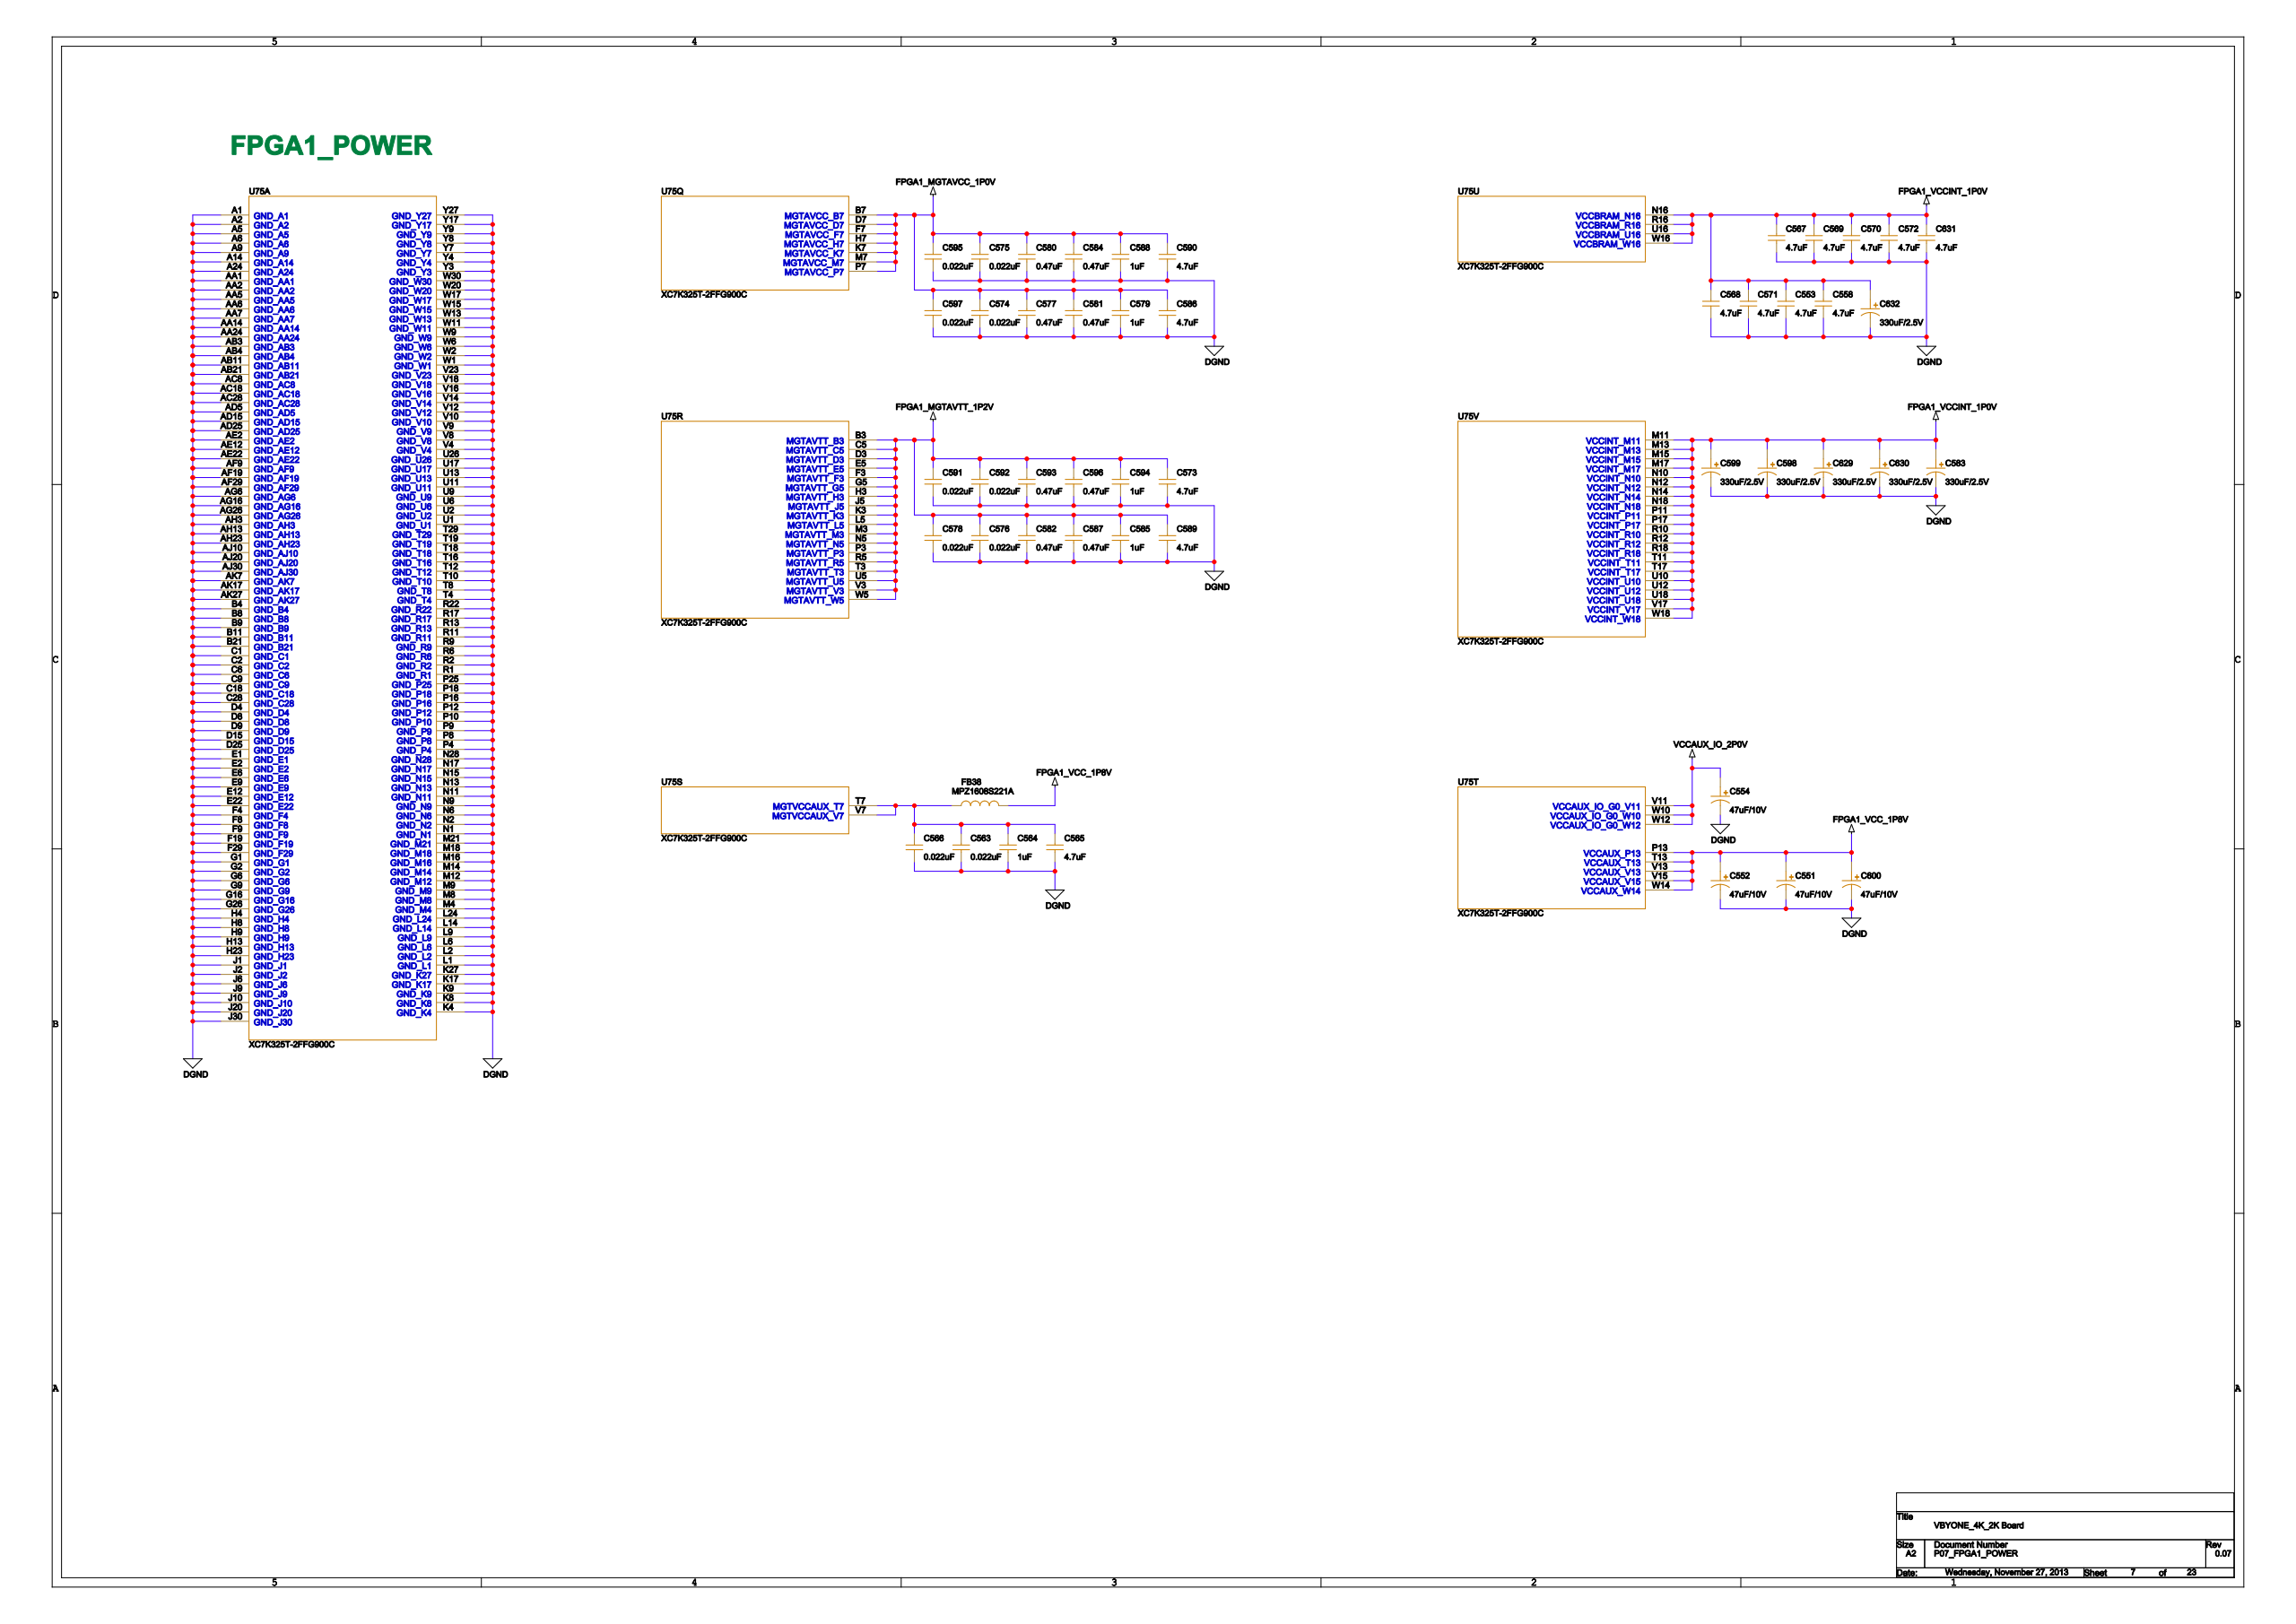Circuit board | Cadence Allegro | 1712 parts | 1495 nets | one sheet of the schematic
Parts on this sheet (reference | value | footprint):
C551 | 47uF/10V | CEC3528RZAS
C552 | 47uF/10V | CEC3528RZAS
C553 | 4.7uF | CRC1608RZAS
C554 | 47uF/10V | CEC3528RZAS
C558 | 4.7uF | CRC1608RZAS
C563 | 0.022uF | CRC1005RZAS
C564 | 1uF | CRC1608RZAS
C565 | 4.7uF | CRC1608RZAS
C566 | 0.022uF | CRC1005RZAS
C567 | 4.7uF | CRC1608RZAS
C568 | 4.7uF | CRC1608RZAS
C569 | 4.7uF | CRC1608RZAS
C570 | 4.7uF | CRC1608RZAS
C571 | 4.7uF | CRC1608RZAS
C572 | 4.7uF | CRC1608RZAS
C573 | 4.7uF | CRC1608RZAS
C574 | 0.022uF | CRC1005RZAS
C575 | 0.022uF | CRC1005RZAS
C576 | 0.022uF | CRC1005RZAS
C577 | 0.47uF | CRC1608RZAS
C578 | 0.022uF | CRC1005RZAS
C579 | 1uF | CRC1608RZAS
C580 | 0.47uF | CRC1608RZAS
C581 | 0.47uF | CRC1608RZAS
C582 | 0.47uF | CRC1608RZAS
C583 | 330uF/2.5V | CEC3528RZAS
C584 | 0.47uF | CRC1608RZAS
C585 | 1uF | CRC1608RZAS
C586 | 4.7uF | CRC1608RZAS
C587 | 0.47uF | CRC1608RZAS
C588 | 1uF | CRC1608RZAS
C589 | 4.7uF | CRC1608RZAS
C590 | 4.7uF | CRC1608RZAS
C591 | 0.022uF | CRC1005RZAS
C592 | 0.022uF | CRC1005RZAS
C593 | 0.47uF | CRC1608RZAS
C594 | 1uF | CRC1608RZAS
C595 | 0.022uF | CRC1005RZAS
C596 | 0.47uF | CRC1608RZAS
C597 | 0.022uF | CRC1005RZAS
C598 | 330uF/2.5V | CEC3528RZAS
C599 | 330uF/2.5V | CEC3528RZAS
C600 | 47uF/10V | CEC3528RZAS
C629 | 330uF/2.5V | CEC3528RZAS
C630 | 330uF/2.5V | CEC3528RZAS
C631 | 4.7uF | CRC1608RZAS
C632 | 330uF/2.5V | CEC3528RZAS
FB38 | MPZ1608S221A | LSC1608RZAS
U9 | SII1161CTU | QFP100RCBS
U10 | SII1161CTU | QFP100RCBS
U16 | SII1161CTU | QFP100RCBS
U26 | K4B4G1646B-HCK0 | BGA096RFDS
U75 | XC7K325T-2FFG900C | BGA900RGAS
Nets of these parts (net: part-pin ...):
DGND: C551-2 C552-2 C553-2 C554-2 C558-2 C563-2 C564-2 C565-2 C566-2 C567-2 C568-2 C569-2 C570-2 C571-2 C572-2 C573-2 C574-2 C575-2 C576-2 C577-2 C578-2 C579-2 C580-2 C581-2 C582-2 C583-2 C584-2 C585-2 C586-2 C587-2 C588-2 C589-2 C590-2 C591-2 C592-2 C593-2 C594-2 C595-2 C596-2 C597-2 C598-2 C599-2 C600-2 C629-2 C630-2 C631-2 C632-2 U9-5 U10-5 U16-5 U26-A9 U26-B3 U26-B9 U26-D8 U26-E1 U26-E2 U26-F9 U26-G1 U26-G9 U26-J2 U26-M9 U26-P9 U75-A1 U75-A2 U75-A5 U75-A6 U75-A9 U75-A14 U75-A24 U75-AA1 U75-AA2 U75-AA5 U75-AA6 U75-AA7 U75-AA14 U75-AA24 U75-AB3 U75-AB4 U75-AB11 U75-AB21 U75-AC8 U75-AC18 U75-AC28 U75-AD5 U75-AD15 U75-AD25 U75-AE2 U75-AE12 U75-AE22 U75-AF9 U75-AF19 U75-AF29 U75-AG6 U75-AG16 U75-AG26 U75-AH3 U75-AH13 U75-AH23 U75-AJ10 U75-AJ20 U75-AJ30 U75-AK7 U75-AK17 U75-AK27 U75-B4 U75-B8 U75-B9 U75-B11 U75-B21 U75-C1 U75-C2 U75-C6 U75-C9 U75-C18 U75-C28 U75-D4 U75-D8 U75-D9 U75-D15 U75-D25 U75-E1 U75-E2 U75-E6 U75-E9 U75-E12 U75-E22 U75-F4 U75-F8 U75-F9 U75-F19 U75-F29 U75-G1 U75-G2 U75-G6 U75-G9 U75-G16 U75-G26 U75-H4 U75-H8 U75-H9 U75-H13 U75-H23 U75-J1 U75-J2 U75-J6 U75-J9 U75-J10 U75-J20 U75-J30 U75-K4 U75-K8 U75-K9 U75-K17 U75-K27 U75-L1 U75-L2 U75-L6 U75-L9 U75-L14 U75-L24 U75-M4 U75-M8 U75-M9 U75-M12 U75-M14 U75-M16 U75-M18 U75-M21 U75-N1 U75-N2 U75-N6 U75-N9 U75-N11 U75-N13 U75-N15 U75-N17 U75-N28 U75-P4 U75-P8 U75-P9 U75-P10 U75-P12 U75-P16 U75-P18 U75-P25 U75-R1 U75-R2 U75-R6 U75-R9 U75-R11 U75-R13 U75-R17 U75-R22 U75-T4 U75-T8 U75-T10 U75-T12 U75-T16 U75-T18 U75-T19 U75-T29 U75-U1 U75-U2 U75-U6 U75-U9 U75-U11 U75-U13 U75-U17 U75-U26 U75-V4 U75-V8 U75-V9 U75-V10 U75-V12 U75-V14 U75-V16 U75-V18 U75-V23 U75-W1 U75-W2 U75-W6 U75-W9 U75-W11 U75-W13 U75-W15 U75-W17 U75-W20 U75-W30 U75-Y3 U75-Y4 U75-Y7 U75-Y8 U75-Y9 U75-Y17 U75-Y27
FPGA1_VCC_1P8V: C551-1 C552-1 C600-1 FB38-2 U75-P13 U75-T13 U75-V13 U75-V15 U75-W14
FPGA1_VCCINT_1P0V: C553-1 C558-1 C567-1 C568-1 C569-1 C570-1 C571-1 C572-1 C583-1 C598-1 C599-1 C629-1 C630-1 C631-1 C632-1 U75-M11 U75-M13 U75-M15 U75-M17 U75-N10 U75-N12 U75-N14 U75-N16 U75-N18 U75-P11 U75-P17 U75-R10 U75-R12 U75-R16 U75-R18 U75-T11 U75-T17 U75-U10 U75-U12 U75-U16 U75-U18 U75-V17 U75-W16 U75-W18
FPGA1_MGTAVTT_1P2V: C573-1 C576-1 C578-1 C582-1 C585-1 C587-1 C589-1 C591-1 C592-1 C593-1 C594-1 C596-1 U75-B3 U75-C5 U75-D3 U75-E5 U75-F3 U75-G5 U75-H3 U75-J5 U75-K3 U75-L5 U75-M3 U75-N5 U75-P3 U75-R5 U75-T3 U75-U5 U75-V3 U75-W5
VCCAUX_IO_2P0V: C554-1 U75-V11 U75-W10 U75-W12
FPGA1_MGTAVCC_1P0V: C574-1 C575-1 C577-1 C579-1 C580-1 C581-1 C584-1 C586-1 C588-1 C590-1 C595-1 C597-1 U75-B7 U75-D7 U75-F7 U75-H7 U75-K7 U75-M7 U75-P7
N16307434: C563-1 C564-1 C565-1 C566-1 FB38-1 U75-T7 U75-V7